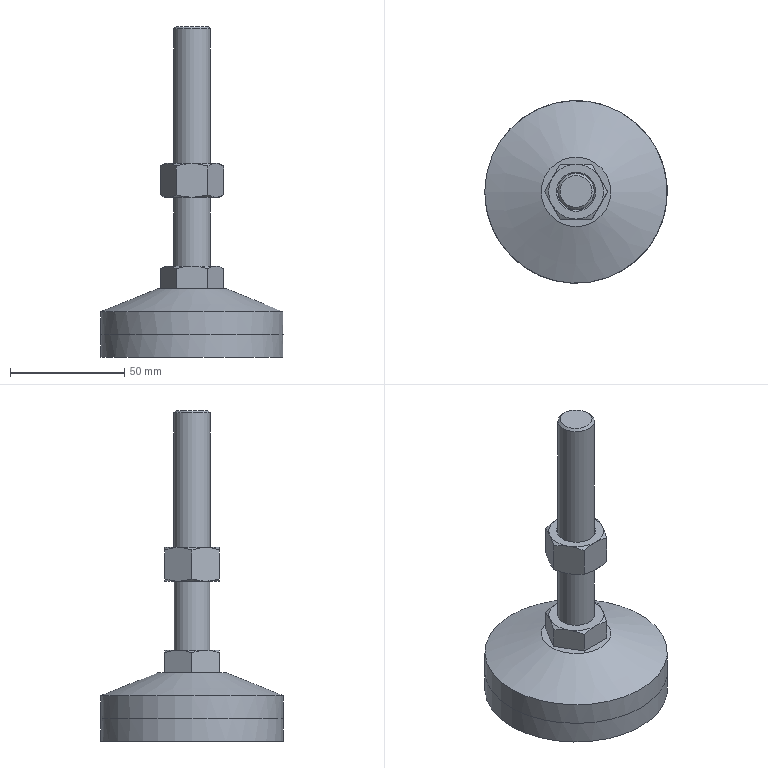Part | STEP file | 冲床-300配套压波_id614_x_t | 1 solid | 44 faces | box 80 x 80 x 145 mm | volume 156529 mm3 | cone 22 | plane 18 | cylinder 4 | commonest cylinder face diameters 16 x2 80 x2
STEP:
#1=CARTESIAN_POINT('',(1145.,255.,-875.));
#2=VERTEX_POINT('',#1);
#3=CARTESIAN_POINT('',(1185.,255.,-875.));
#4=DIRECTION('',(0.,0.,1.));
#5=DIRECTION('',(-1.,0.,0.));
#6=AXIS2_PLACEMENT_3D('',#3,#4,#5);
#7=CIRCLE('',#6,40.);
#8=EDGE_CURVE('',#2,#2,#7,.T.);
#9=ORIENTED_EDGE('',*,*,#8,.T.);
#10=EDGE_LOOP('',(#9));
#11=FACE_BOUND('',#10,.T.);
#12=CARTESIAN_POINT('',(1145.,255.,-865.));
#13=VERTEX_POINT('',#12);
#14=CARTESIAN_POINT('',(1145.,249.764,-865.));
#15=CARTESIAN_POINT('',(1145.,260.236,-865.));
#16=CARTESIAN_POINT('',(1146.041,265.47,-865.));
#17=CARTESIAN_POINT('',(1150.049,275.145,-865.));
#18=CARTESIAN_POINT('',(1153.013,279.582,-865.));
#19=CARTESIAN_POINT('',(1160.418,286.987,-865.));
#20=CARTESIAN_POINT('',(1164.855,289.951,-865.));
#21=CARTESIAN_POINT('',(1174.53,293.959,-865.));
#22=CARTESIAN_POINT('',(1179.764,295.,-865.));
#23=CARTESIAN_POINT('',(1190.236,295.,-865.));
#24=CARTESIAN_POINT('',(1195.47,293.959,-865.));
#25=CARTESIAN_POINT('',(1205.145,289.951,-865.));
#26=CARTESIAN_POINT('',(1209.582,286.987,-865.));
#27=CARTESIAN_POINT('',(1216.987,279.582,-865.));
#28=CARTESIAN_POINT('',(1219.951,275.145,-865.));
#29=CARTESIAN_POINT('',(1223.959,265.47,-865.));
#30=CARTESIAN_POINT('',(1225.,260.236,-865.));
#31=CARTESIAN_POINT('',(1225.,249.764,-865.));
#32=CARTESIAN_POINT('',(1223.959,244.53,-865.));
#33=CARTESIAN_POINT('',(1219.951,234.855,-865.));
#34=CARTESIAN_POINT('',(1216.987,230.418,-865.));
#35=CARTESIAN_POINT('',(1209.582,223.013,-865.));
#36=CARTESIAN_POINT('',(1205.145,220.049,-865.));
#37=CARTESIAN_POINT('',(1195.47,216.041,-865.));
#38=CARTESIAN_POINT('',(1190.236,215.,-865.));
#39=CARTESIAN_POINT('',(1179.764,215.,-865.));
#40=CARTESIAN_POINT('',(1174.53,216.041,-865.));
#41=CARTESIAN_POINT('',(1164.855,220.049,-865.));
#42=CARTESIAN_POINT('',(1160.418,223.013,-865.));
#43=CARTESIAN_POINT('',(1153.013,230.418,-865.));
#44=CARTESIAN_POINT('',(1150.049,234.855,-865.));
#45=CARTESIAN_POINT('',(1146.041,244.53,-865.));
#46=CARTESIAN_POINT('',(1145.,249.764,-865.));
#47=CARTESIAN_POINT('',(1145.,260.236,-865.));
#48=B_SPLINE_CURVE_WITH_KNOTS('',3,(#14,#15,#16,#17,#18,#19,#20,#21,#22,#23,#24,#25,#26,#27,#28,#29,#30,#31,#32,#33,#34,#35,#36,#37,#38,#39,#40,#41,#42,#43,#44,#45,#46,#47),.UNSPECIFIED.,.T.,.F.,(2,2,2,2,2,2,2,2,2,2,2,2,2,2,2,2,2,2,2),(-0.0625,0.,0.0625,0.125,0.1875,0.25,0.3125,0.375,0.4375,0.5,0.5625,0.625,0.6875,0.75,0.8125,0.875,0.9375,1.,1.062),.UNSPECIFIED.);
#49=EDGE_CURVE('',#13,#13,#48,.T.);
#50=ORIENTED_EDGE('',*,*,#49,.T.);
#51=EDGE_LOOP('',(#50));
#52=FACE_BOUND('',#51,.T.);
#53=CARTESIAN_POINT('',(1185.,255.,-855.));
#54=DIRECTION('',(0.,0.,-1.));
#55=DIRECTION('',(-1.,0.,0.));
#56=AXIS2_PLACEMENT_3D('',#53,#54,#55);
#57=CYLINDRICAL_SURFACE('',#56,40.);
#58=ADVANCED_FACE('',(#11,#52),#57,.T.);
#59=ORIENTED_EDGE('',*,*,#49,.F.);
#60=EDGE_LOOP('',(#59));
#61=FACE_BOUND('',#60,.T.);
#62=CARTESIAN_POINT('',(1145.,255.,-855.));
#63=VERTEX_POINT('',#62);
#64=CARTESIAN_POINT('',(1185.,255.,-855.));
#65=DIRECTION('',(0.,0.,1.));
#66=DIRECTION('',(-1.,0.,0.));
#67=AXIS2_PLACEMENT_3D('',#64,#65,#66);
#68=CIRCLE('',#67,40.);
#69=EDGE_CURVE('',#63,#63,#68,.T.);
#70=ORIENTED_EDGE('',*,*,#69,.F.);
#71=EDGE_LOOP('',(#70));
#72=FACE_BOUND('',#71,.T.);
#73=CARTESIAN_POINT('',(1185.,255.,-855.));
#74=DIRECTION('',(0.,0.,-1.));
#75=DIRECTION('',(-1.,0.,0.));
#76=AXIS2_PLACEMENT_3D('',#73,#74,#75);
#77=CYLINDRICAL_SURFACE('',#76,40.);
#78=ADVANCED_FACE('',(#61,#72),#77,.T.);
#79=ORIENTED_EDGE('',*,*,#8,.F.);
#80=EDGE_LOOP('',(#79));
#81=FACE_OUTER_BOUND('',#80,.T.);
#82=CARTESIAN_POINT('',(1185.,255.,-875.));
#83=DIRECTION('',(0.,0.,1.));
#84=DIRECTION('',(1.,0.,0.));
#85=AXIS2_PLACEMENT_3D('',#82,#83,#84);
#86=PLANE('',#85);
#87=ADVANCED_FACE('',(#81),#86,.F.);
#88=CARTESIAN_POINT('',(1169.751,255.,-845.));
#89=VERTEX_POINT('',#88);
#90=CARTESIAN_POINT('',(1185.,255.,-845.));
#91=DIRECTION('',(0.,0.,-1.));
#92=DIRECTION('',(-1.,0.,0.));
#93=AXIS2_PLACEMENT_3D('',#90,#91,#92);
#94=CIRCLE('',#93,15.249);
#95=EDGE_CURVE('',#89,#89,#94,.T.);
#96=ORIENTED_EDGE('',*,*,#95,.T.);
#97=EDGE_LOOP('',(#96));
#98=FACE_BOUND('',#97,.T.);
#99=ORIENTED_EDGE('',*,*,#69,.T.);
#100=EDGE_LOOP('',(#99));
#101=FACE_BOUND('',#100,.T.);
#102=CARTESIAN_POINT('',(1185.,255.,-855.));
#103=DIRECTION('',(0.,0.,-1.));
#104=DIRECTION('',(-1.,0.,0.));
#105=AXIS2_PLACEMENT_3D('',#102,#103,#104);
#106=CONICAL_SURFACE('',#105,40.,68.);
#107=ADVANCED_FACE('',(#98,#101),#106,.T.);
#108=CARTESIAN_POINT('',(1191.928,243.,-845.));
#109=VERTEX_POINT('',#108);
#110=CARTESIAN_POINT('',(1198.856,255.,-845.));
#111=VERTEX_POINT('',#110);
#112=CARTESIAN_POINT('',(1191.928,243.,-845.));
#113=DIRECTION('',(0.5,0.866,0.));
#114=VECTOR('',#113,1.);
#115=LINE('',#112,#114);
#116=EDGE_CURVE('',#109,#111,#115,.T.);
#117=ORIENTED_EDGE('',*,*,#116,.F.);
#118=CARTESIAN_POINT('',(1178.072,243.,-845.));
#119=VERTEX_POINT('',#118);
#120=CARTESIAN_POINT('',(1178.072,243.,-845.));
#121=DIRECTION('',(1.,0.,0.));
#122=VECTOR('',#121,1.);
#123=LINE('',#120,#122);
#124=EDGE_CURVE('',#119,#109,#123,.T.);
#125=ORIENTED_EDGE('',*,*,#124,.F.);
#126=CARTESIAN_POINT('',(1171.144,255.,-845.));
#127=VERTEX_POINT('',#126);
#128=CARTESIAN_POINT('',(1171.144,255.,-845.));
#129=DIRECTION('',(0.5,-0.866,0.));
#130=VECTOR('',#129,1.);
#131=LINE('',#128,#130);
#132=EDGE_CURVE('',#127,#119,#131,.T.);
#133=ORIENTED_EDGE('',*,*,#132,.F.);
#134=CARTESIAN_POINT('',(1178.072,267.,-845.));
#135=VERTEX_POINT('',#134);
#136=CARTESIAN_POINT('',(1178.072,267.,-845.));
#137=DIRECTION('',(-0.5,-0.866,0.));
#138=VECTOR('',#137,1.);
#139=LINE('',#136,#138);
#140=EDGE_CURVE('',#135,#127,#139,.T.);
#141=ORIENTED_EDGE('',*,*,#140,.F.);
#142=CARTESIAN_POINT('',(1191.928,267.,-845.));
#143=VERTEX_POINT('',#142);
#144=CARTESIAN_POINT('',(1191.928,267.,-845.));
#145=DIRECTION('',(-1.,0.,0.));
#146=VECTOR('',#145,1.);
#147=LINE('',#144,#146);
#148=EDGE_CURVE('',#143,#135,#147,.T.);
#149=ORIENTED_EDGE('',*,*,#148,.F.);
#150=CARTESIAN_POINT('',(1198.856,255.,-845.));
#151=DIRECTION('',(-0.5,0.866,0.));
#152=VECTOR('',#151,1.);
#153=LINE('',#150,#152);
#154=EDGE_CURVE('',#111,#143,#153,.T.);
#155=ORIENTED_EDGE('',*,*,#154,.F.);
#156=EDGE_LOOP('',(#117,#125,#133,#141,#149,#155));
#157=FACE_BOUND('',#156,.T.);
#158=ORIENTED_EDGE('',*,*,#95,.F.);
#159=EDGE_LOOP('',(#158));
#160=FACE_BOUND('',#159,.T.);
#161=CARTESIAN_POINT('',(1185.,255.,-845.));
#162=DIRECTION('',(0.,0.,-1.));
#163=DIRECTION('',(-1.,0.,0.));
#164=AXIS2_PLACEMENT_3D('',#161,#162,#163);
#165=PLANE('',#164);
#166=ADVANCED_FACE('',(#157,#160),#165,.F.);
#167=CARTESIAN_POINT('',(1178.072,243.,-836.072));
#168=VERTEX_POINT('',#167);
#169=CARTESIAN_POINT('',(1178.072,243.,-830.2));
#170=DIRECTION('',(0.,0.,1.));
#171=VECTOR('',#170,1.);
#172=LINE('',#169,#171);
#173=EDGE_CURVE('',#119,#168,#172,.T.);
#174=ORIENTED_EDGE('',*,*,#173,.T.);
#175=CARTESIAN_POINT('',(1174.608,249.,-835.));
#176=VERTEX_POINT('',#175);
#177=CARTESIAN_POINT('',(1174.608,249.,-835.));
#178=CARTESIAN_POINT('',(1175.788,246.956,-835.));
#179=CARTESIAN_POINT('',(1176.938,244.963,-835.417));
#180=CARTESIAN_POINT('',(1178.072,243.,-836.072));
#181=B_SPLINE_CURVE_WITH_KNOTS('',3,(#177,#178,#179,#180),.UNSPECIFIED.,.F.,.F.,(4,4),(0.,1.),.UNSPECIFIED.);
#182=EDGE_CURVE('',#176,#168,#181,.T.);
#183=ORIENTED_EDGE('',*,*,#182,.F.);
#184=CARTESIAN_POINT('',(1171.144,255.,-836.072));
#185=VERTEX_POINT('',#184);
#186=CARTESIAN_POINT('',(1171.144,255.,-836.072));
#187=CARTESIAN_POINT('',(1172.277,253.037,-835.417));
#188=CARTESIAN_POINT('',(1173.427,251.044,-835.));
#189=CARTESIAN_POINT('',(1174.608,249.,-835.));
#190=B_SPLINE_CURVE_WITH_KNOTS('',3,(#186,#187,#188,#189),.UNSPECIFIED.,.F.,.F.,(4,4),(0.,1.),.UNSPECIFIED.);
#191=EDGE_CURVE('',#185,#176,#190,.T.);
#192=ORIENTED_EDGE('',*,*,#191,.F.);
#193=CARTESIAN_POINT('',(1171.144,255.,-830.2));
#194=DIRECTION('',(0.,0.,1.));
#195=VECTOR('',#194,1.);
#196=LINE('',#193,#195);
#197=EDGE_CURVE('',#127,#185,#196,.T.);
#198=ORIENTED_EDGE('',*,*,#197,.F.);
#199=ORIENTED_EDGE('',*,*,#132,.T.);
#200=EDGE_LOOP('',(#174,#183,#192,#198,#199));
#201=FACE_OUTER_BOUND('',#200,.T.);
#202=CARTESIAN_POINT('',(1171.144,255.,-830.2));
#203=DIRECTION('',(-0.866,-0.5,0.));
#204=DIRECTION('',(-0.5,0.866,0.));
#205=AXIS2_PLACEMENT_3D('',#202,#203,#204);
#206=PLANE('',#205);
#207=ADVANCED_FACE('',(#201),#206,.T.);
#208=CARTESIAN_POINT('',(1191.928,243.,-836.072));
#209=VERTEX_POINT('',#208);
#210=CARTESIAN_POINT('',(1191.928,243.,-830.2));
#211=DIRECTION('',(0.,0.,1.));
#212=VECTOR('',#211,1.);
#213=LINE('',#210,#212);
#214=EDGE_CURVE('',#109,#209,#213,.T.);
#215=ORIENTED_EDGE('',*,*,#214,.T.);
#216=CARTESIAN_POINT('',(1185.,243.,-835.));
#217=VERTEX_POINT('',#216);
#218=CARTESIAN_POINT('',(1185.,243.,-835.));
#219=CARTESIAN_POINT('',(1187.361,243.,-835.));
#220=CARTESIAN_POINT('',(1189.661,243.,-835.417));
#221=CARTESIAN_POINT('',(1191.928,243.,-836.072));
#222=B_SPLINE_CURVE_WITH_KNOTS('',3,(#218,#219,#220,#221),.UNSPECIFIED.,.F.,.F.,(4,4),(0.,1.),.UNSPECIFIED.);
#223=EDGE_CURVE('',#217,#209,#222,.T.);
#224=ORIENTED_EDGE('',*,*,#223,.F.);
#225=CARTESIAN_POINT('',(1178.072,243.,-836.072));
#226=CARTESIAN_POINT('',(1180.339,243.,-835.417));
#227=CARTESIAN_POINT('',(1182.639,243.,-835.));
#228=CARTESIAN_POINT('',(1185.,243.,-835.));
#229=B_SPLINE_CURVE_WITH_KNOTS('',3,(#225,#226,#227,#228),.UNSPECIFIED.,.F.,.F.,(4,4),(0.,1.),.UNSPECIFIED.);
#230=EDGE_CURVE('',#168,#217,#229,.T.);
#231=ORIENTED_EDGE('',*,*,#230,.F.);
#232=ORIENTED_EDGE('',*,*,#173,.F.);
#233=ORIENTED_EDGE('',*,*,#124,.T.);
#234=EDGE_LOOP('',(#215,#224,#231,#232,#233));
#235=FACE_OUTER_BOUND('',#234,.T.);
#236=CARTESIAN_POINT('',(1178.072,243.,-830.2));
#237=DIRECTION('',(0.,-1.,0.));
#238=DIRECTION('',(0.,0.,1.));
#239=AXIS2_PLACEMENT_3D('',#236,#237,#238);
#240=PLANE('',#239);
#241=ADVANCED_FACE('',(#235),#240,.T.);
#242=CARTESIAN_POINT('',(1198.856,255.,-836.072));
#243=VERTEX_POINT('',#242);
#244=CARTESIAN_POINT('',(1198.856,255.,-830.2));
#245=DIRECTION('',(0.,0.,1.));
#246=VECTOR('',#245,1.);
#247=LINE('',#244,#246);
#248=EDGE_CURVE('',#111,#243,#247,.T.);
#249=ORIENTED_EDGE('',*,*,#248,.T.);
#250=CARTESIAN_POINT('',(1195.392,249.,-835.));
#251=VERTEX_POINT('',#250);
#252=CARTESIAN_POINT('',(1195.392,249.,-835.));
#253=CARTESIAN_POINT('',(1196.573,251.044,-835.));
#254=CARTESIAN_POINT('',(1197.723,253.037,-835.417));
#255=CARTESIAN_POINT('',(1198.856,255.,-836.072));
#256=B_SPLINE_CURVE_WITH_KNOTS('',3,(#252,#253,#254,#255),.UNSPECIFIED.,.F.,.F.,(4,4),(0.,1.),.UNSPECIFIED.);
#257=EDGE_CURVE('',#251,#243,#256,.T.);
#258=ORIENTED_EDGE('',*,*,#257,.F.);
#259=CARTESIAN_POINT('',(1191.928,243.,-836.072));
#260=CARTESIAN_POINT('',(1193.062,244.963,-835.417));
#261=CARTESIAN_POINT('',(1194.212,246.956,-835.));
#262=CARTESIAN_POINT('',(1195.392,249.,-835.));
#263=B_SPLINE_CURVE_WITH_KNOTS('',3,(#259,#260,#261,#262),.UNSPECIFIED.,.F.,.F.,(4,4),(0.,1.),.UNSPECIFIED.);
#264=EDGE_CURVE('',#209,#251,#263,.T.);
#265=ORIENTED_EDGE('',*,*,#264,.F.);
#266=ORIENTED_EDGE('',*,*,#214,.F.);
#267=ORIENTED_EDGE('',*,*,#116,.T.);
#268=EDGE_LOOP('',(#249,#258,#265,#266,#267));
#269=FACE_OUTER_BOUND('',#268,.T.);
#270=CARTESIAN_POINT('',(1191.928,243.,-830.2));
#271=DIRECTION('',(0.866,-0.5,0.));
#272=DIRECTION('',(-0.5,-0.866,0.));
#273=AXIS2_PLACEMENT_3D('',#270,#271,#272);
#274=PLANE('',#273);
#275=ADVANCED_FACE('',(#269),#274,.T.);
#276=CARTESIAN_POINT('',(1191.928,267.,-836.072));
#277=VERTEX_POINT('',#276);
#278=CARTESIAN_POINT('',(1191.928,267.,-830.2));
#279=DIRECTION('',(0.,0.,1.));
#280=VECTOR('',#279,1.);
#281=LINE('',#278,#280);
#282=EDGE_CURVE('',#143,#277,#281,.T.);
#283=ORIENTED_EDGE('',*,*,#282,.T.);
#284=CARTESIAN_POINT('',(1195.392,261.,-835.));
#285=VERTEX_POINT('',#284);
#286=CARTESIAN_POINT('',(1195.392,261.,-835.));
#287=CARTESIAN_POINT('',(1194.212,263.044,-835.));
#288=CARTESIAN_POINT('',(1193.062,265.037,-835.417));
#289=CARTESIAN_POINT('',(1191.928,267.,-836.072));
#290=B_SPLINE_CURVE_WITH_KNOTS('',3,(#286,#287,#288,#289),.UNSPECIFIED.,.F.,.F.,(4,4),(0.,1.),.UNSPECIFIED.);
#291=EDGE_CURVE('',#285,#277,#290,.T.);
#292=ORIENTED_EDGE('',*,*,#291,.F.);
#293=CARTESIAN_POINT('',(1198.856,255.,-836.072));
#294=CARTESIAN_POINT('',(1197.723,256.963,-835.417));
#295=CARTESIAN_POINT('',(1196.573,258.956,-835.));
#296=CARTESIAN_POINT('',(1195.392,261.,-835.));
#297=B_SPLINE_CURVE_WITH_KNOTS('',3,(#293,#294,#295,#296),.UNSPECIFIED.,.F.,.F.,(4,4),(0.,1.),.UNSPECIFIED.);
#298=EDGE_CURVE('',#243,#285,#297,.T.);
#299=ORIENTED_EDGE('',*,*,#298,.F.);
#300=ORIENTED_EDGE('',*,*,#248,.F.);
#301=ORIENTED_EDGE('',*,*,#154,.T.);
#302=EDGE_LOOP('',(#283,#292,#299,#300,#301));
#303=FACE_OUTER_BOUND('',#302,.T.);
#304=CARTESIAN_POINT('',(1198.856,255.,-830.2));
#305=DIRECTION('',(0.866,0.5,0.));
#306=DIRECTION('',(0.5,-0.866,0.));
#307=AXIS2_PLACEMENT_3D('',#304,#305,#306);
#308=PLANE('',#307);
#309=ADVANCED_FACE('',(#303),#308,.T.);
#310=CARTESIAN_POINT('',(1178.072,267.,-836.072));
#311=VERTEX_POINT('',#310);
#312=CARTESIAN_POINT('',(1178.072,267.,-830.2));
#313=DIRECTION('',(0.,0.,1.));
#314=VECTOR('',#313,1.);
#315=LINE('',#312,#314);
#316=EDGE_CURVE('',#135,#311,#315,.T.);
#317=ORIENTED_EDGE('',*,*,#316,.T.);
#318=CARTESIAN_POINT('',(1185.,267.,-835.));
#319=VERTEX_POINT('',#318);
#320=CARTESIAN_POINT('',(1185.,267.,-835.));
#321=CARTESIAN_POINT('',(1182.639,267.,-835.));
#322=CARTESIAN_POINT('',(1180.339,267.,-835.417));
#323=CARTESIAN_POINT('',(1178.072,267.,-836.072));
#324=B_SPLINE_CURVE_WITH_KNOTS('',3,(#320,#321,#322,#323),.UNSPECIFIED.,.F.,.F.,(4,4),(0.,1.),.UNSPECIFIED.);
#325=EDGE_CURVE('',#319,#311,#324,.T.);
#326=ORIENTED_EDGE('',*,*,#325,.F.);
#327=CARTESIAN_POINT('',(1191.928,267.,-836.072));
#328=CARTESIAN_POINT('',(1189.661,267.,-835.417));
#329=CARTESIAN_POINT('',(1187.361,267.,-835.));
#330=CARTESIAN_POINT('',(1185.,267.,-835.));
#331=B_SPLINE_CURVE_WITH_KNOTS('',3,(#327,#328,#329,#330),.UNSPECIFIED.,.F.,.F.,(4,4),(0.,1.),.UNSPECIFIED.);
#332=EDGE_CURVE('',#277,#319,#331,.T.);
#333=ORIENTED_EDGE('',*,*,#332,.F.);
#334=ORIENTED_EDGE('',*,*,#282,.F.);
#335=ORIENTED_EDGE('',*,*,#148,.T.);
#336=EDGE_LOOP('',(#317,#326,#333,#334,#335));
#337=FACE_OUTER_BOUND('',#336,.T.);
#338=CARTESIAN_POINT('',(1191.928,267.,-830.2));
#339=DIRECTION('',(0.,1.,0.));
#340=DIRECTION('',(0.,0.,-1.));
#341=AXIS2_PLACEMENT_3D('',#338,#339,#340);
#342=PLANE('',#341);
#343=ADVANCED_FACE('',(#337),#342,.T.);
#344=ORIENTED_EDGE('',*,*,#197,.T.);
#345=CARTESIAN_POINT('',(1174.608,261.,-835.));
#346=VERTEX_POINT('',#345);
#347=CARTESIAN_POINT('',(1174.608,261.,-835.));
#348=CARTESIAN_POINT('',(1173.427,258.956,-835.));
#349=CARTESIAN_POINT('',(1172.277,256.963,-835.417));
#350=CARTESIAN_POINT('',(1171.144,255.,-836.072));
#351=B_SPLINE_CURVE_WITH_KNOTS('',3,(#347,#348,#349,#350),.UNSPECIFIED.,.F.,.F.,(4,4),(0.,1.),.UNSPECIFIED.);
#352=EDGE_CURVE('',#346,#185,#351,.T.);
#353=ORIENTED_EDGE('',*,*,#352,.F.);
#354=CARTESIAN_POINT('',(1178.072,267.,-836.072));
#355=CARTESIAN_POINT('',(1176.938,265.037,-835.417));
#356=CARTESIAN_POINT('',(1175.788,263.044,-835.));
#357=CARTESIAN_POINT('',(1174.608,261.,-835.));
#358=B_SPLINE_CURVE_WITH_KNOTS('',3,(#354,#355,#356,#357),.UNSPECIFIED.,.F.,.F.,(4,4),(0.,1.),.UNSPECIFIED.);
#359=EDGE_CURVE('',#311,#346,#358,.T.);
#360=ORIENTED_EDGE('',*,*,#359,.F.);
#361=ORIENTED_EDGE('',*,*,#316,.F.);
#362=ORIENTED_EDGE('',*,*,#140,.T.);
#363=EDGE_LOOP('',(#344,#353,#360,#361,#362));
#364=FACE_OUTER_BOUND('',#363,.T.);
#365=CARTESIAN_POINT('',(1178.072,267.,-830.2));
#366=DIRECTION('',(-0.866,0.5,0.));
#367=DIRECTION('',(0.5,0.866,0.));
#368=AXIS2_PLACEMENT_3D('',#365,#366,#367);
#369=PLANE('',#368);
#370=ADVANCED_FACE('',(#364),#369,.T.);
#371=CARTESIAN_POINT('',(1177.,255.,-835.));
#372=VERTEX_POINT('',#371);
#373=CARTESIAN_POINT('',(1185.,255.,-835.));
#374=DIRECTION('',(0.,0.,1.));
#375=DIRECTION('',(-1.,0.,0.));
#376=AXIS2_PLACEMENT_3D('',#373,#374,#375);
#377=CIRCLE('',#376,8.);
#378=EDGE_CURVE('',#372,#372,#377,.T.);
#379=ORIENTED_EDGE('',*,*,#378,.F.);
#380=EDGE_LOOP('',(#379));
#381=FACE_BOUND('',#380,.T.);
#382=CARTESIAN_POINT('',(1185.,255.,-835.));
#383=DIRECTION('',(0.,0.,-1.));
#384=DIRECTION('',(-1.,0.,0.));
#385=AXIS2_PLACEMENT_3D('',#382,#383,#384);
#386=CIRCLE('',#385,12.);
#387=EDGE_CURVE('',#217,#176,#386,.T.);
#388=ORIENTED_EDGE('',*,*,#387,.F.);
#389=CARTESIAN_POINT('',(1185.,255.,-835.));
#390=DIRECTION('',(0.,0.,-1.));
#391=DIRECTION('',(-1.,0.,0.));
#392=AXIS2_PLACEMENT_3D('',#389,#390,#391);
#393=CIRCLE('',#392,12.);
#394=EDGE_CURVE('',#251,#217,#393,.T.);
#395=ORIENTED_EDGE('',*,*,#394,.F.);
#396=CARTESIAN_POINT('',(1185.,255.,-835.));
#397=DIRECTION('',(0.,0.,-1.));
#398=DIRECTION('',(-1.,0.,0.));
#399=AXIS2_PLACEMENT_3D('',#396,#397,#398);
#400=CIRCLE('',#399,12.);
#401=EDGE_CURVE('',#285,#251,#400,.T.);
#402=ORIENTED_EDGE('',*,*,#401,.F.);
#403=CARTESIAN_POINT('',(1185.,255.,-835.));
#404=DIRECTION('',(0.,0.,-1.));
#405=DIRECTION('',(-1.,0.,0.));
#406=AXIS2_PLACEMENT_3D('',#403,#404,#405);
#407=CIRCLE('',#406,12.);
#408=EDGE_CURVE('',#319,#285,#407,.T.);
#409=ORIENTED_EDGE('',*,*,#408,.F.);
#410=CARTESIAN_POINT('',(1185.,255.,-835.));
#411=DIRECTION('',(0.,0.,-1.));
#412=DIRECTION('',(-1.,0.,0.));
#413=AXIS2_PLACEMENT_3D('',#410,#411,#412);
#414=CIRCLE('',#413,12.);
#415=EDGE_CURVE('',#346,#319,#414,.T.);
#416=ORIENTED_EDGE('',*,*,#415,.F.);
#417=CARTESIAN_POINT('',(1185.,255.,-835.));
#418=DIRECTION('',(0.,0.,-1.));
#419=DIRECTION('',(-1.,0.,0.));
#420=AXIS2_PLACEMENT_3D('',#417,#418,#419);
#421=CIRCLE('',#420,12.);
#422=EDGE_CURVE('',#176,#346,#421,.T.);
#423=ORIENTED_EDGE('',*,*,#422,.F.);
#424=EDGE_LOOP('',(#388,#395,#402,#409,#416,#423));
#425=FACE_BOUND('',#424,.T.);
#426=CARTESIAN_POINT('',(1178.072,243.,-835.));
#427=DIRECTION('',(0.,0.,-1.));
#428=DIRECTION('',(-1.,0.,0.));
#429=AXIS2_PLACEMENT_3D('',#426,#427,#428);
#430=PLANE('',#429);
#431=ADVANCED_FACE('',(#381,#425),#430,.F.);
#432=ORIENTED_EDGE('',*,*,#325,.T.);
#433=ORIENTED_EDGE('',*,*,#359,.T.);
#434=ORIENTED_EDGE('',*,*,#415,.T.);
#435=EDGE_LOOP('',(#432,#433,#434));
#436=FACE_OUTER_BOUND('',#435,.T.);
#437=CARTESIAN_POINT('',(1185.,255.,-835.));
#438=DIRECTION('',(0.,0.,-1.));
#439=DIRECTION('',(-1.,0.,0.));
#440=AXIS2_PLACEMENT_3D('',#437,#438,#439);
#441=CONICAL_SURFACE('',#440,12.,60.);
#442=ADVANCED_FACE('',(#436),#441,.T.);
#443=ORIENTED_EDGE('',*,*,#191,.T.);
#444=ORIENTED_EDGE('',*,*,#422,.T.);
#445=ORIENTED_EDGE('',*,*,#352,.T.);
#446=EDGE_LOOP('',(#443,#444,#445));
#447=FACE_OUTER_BOUND('',#446,.T.);
#448=CARTESIAN_POINT('',(1185.,255.,-835.));
#449=DIRECTION('',(0.,0.,-1.));
#450=DIRECTION('',(-1.,0.,0.));
#451=AXIS2_PLACEMENT_3D('',#448,#449,#450);
#452=CONICAL_SURFACE('',#451,12.,60.);
#453=ADVANCED_FACE('',(#447),#452,.T.);
#454=ORIENTED_EDGE('',*,*,#291,.T.);
#455=ORIENTED_EDGE('',*,*,#332,.T.);
#456=ORIENTED_EDGE('',*,*,#408,.T.);
#457=EDGE_LOOP('',(#454,#455,#456));
#458=FACE_OUTER_BOUND('',#457,.T.);
#459=CARTESIAN_POINT('',(1185.,255.,-835.));
#460=DIRECTION('',(0.,0.,-1.));
#461=DIRECTION('',(-1.,0.,0.));
#462=AXIS2_PLACEMENT_3D('',#459,#460,#461);
#463=CONICAL_SURFACE('',#462,12.,60.);
#464=ADVANCED_FACE('',(#458),#463,.T.);
#465=ORIENTED_EDGE('',*,*,#257,.T.);
#466=ORIENTED_EDGE('',*,*,#298,.T.);
#467=ORIENTED_EDGE('',*,*,#401,.T.);
#468=EDGE_LOOP('',(#465,#466,#467));
#469=FACE_OUTER_BOUND('',#468,.T.);
#470=CARTESIAN_POINT('',(1185.,255.,-835.));
#471=DIRECTION('',(0.,0.,-1.));
#472=DIRECTION('',(-1.,0.,0.));
#473=AXIS2_PLACEMENT_3D('',#470,#471,#472);
#474=CONICAL_SURFACE('',#473,12.,60.);
#475=ADVANCED_FACE('',(#469),#474,.T.);
#476=ORIENTED_EDGE('',*,*,#264,.T.);
#477=ORIENTED_EDGE('',*,*,#394,.T.);
#478=ORIENTED_EDGE('',*,*,#223,.T.);
#479=EDGE_LOOP('',(#476,#477,#478));
#480=FACE_OUTER_BOUND('',#479,.T.);
#481=CARTESIAN_POINT('',(1185.,255.,-835.));
#482=DIRECTION('',(0.,0.,-1.));
#483=DIRECTION('',(-1.,0.,0.));
#484=AXIS2_PLACEMENT_3D('',#481,#482,#483);
#485=CONICAL_SURFACE('',#484,12.,60.);
#486=ADVANCED_FACE('',(#480),#485,.T.);
#487=ORIENTED_EDGE('',*,*,#230,.T.);
#488=ORIENTED_EDGE('',*,*,#387,.T.);
#489=ORIENTED_EDGE('',*,*,#182,.T.);
#490=EDGE_LOOP('',(#487,#488,#489));
#491=FACE_OUTER_BOUND('',#490,.T.);
#492=CARTESIAN_POINT('',(1185.,255.,-835.));
#493=DIRECTION('',(0.,0.,-1.));
#494=DIRECTION('',(-1.,0.,0.));
#495=AXIS2_PLACEMENT_3D('',#492,#493,#494);
#496=CONICAL_SURFACE('',#495,12.,60.);
#497=ADVANCED_FACE('',(#491),#496,.T.);
#498=CARTESIAN_POINT('',(1177.,255.,-804.232));
#499=VERTEX_POINT('',#498);
#500=CARTESIAN_POINT('',(1185.,255.,-804.232));
#501=DIRECTION('',(0.,0.,1.));
#502=DIRECTION('',(-1.,0.,0.));
#503=AXIS2_PLACEMENT_3D('',#500,#501,#502);
#504=CIRCLE('',#503,8.);
#505=EDGE_CURVE('',#499,#499,#504,.T.);
#506=ORIENTED_EDGE('',*,*,#505,.F.);
#507=EDGE_LOOP('',(#506));
#508=FACE_BOUND('',#507,.T.);
#509=ORIENTED_EDGE('',*,*,#378,.T.);
#510=EDGE_LOOP('',(#509));
#511=FACE_BOUND('',#510,.T.);
#512=CARTESIAN_POINT('',(1185.,255.,-740.));
#513=DIRECTION('',(0.,0.,-1.));
#514=DIRECTION('',(-1.,0.,0.));
#515=AXIS2_PLACEMENT_3D('',#512,#513,#514);
#516=CYLINDRICAL_SURFACE('',#515,8.);
#517=ADVANCED_FACE('',(#508,#511),#516,.T.);
#518=CARTESIAN_POINT('',(1191.928,243.,-791.072));
#519=VERTEX_POINT('',#518);
#520=CARTESIAN_POINT('',(1191.928,243.,-803.728));
#521=VERTEX_POINT('',#520);
#522=CARTESIAN_POINT('',(1191.928,243.,-804.8));
#523=DIRECTION('',(0.,0.,-1.));
#524=VECTOR('',#523,1.);
#525=LINE('',#522,#524);
#526=EDGE_CURVE('',#519,#521,#525,.T.);
#527=ORIENTED_EDGE('',*,*,#526,.T.);
#528=CARTESIAN_POINT('',(1195.392,249.,-804.8));
#529=VERTEX_POINT('',#528);
#530=CARTESIAN_POINT('',(1195.392,249.,-804.8));
#531=CARTESIAN_POINT('',(1194.212,246.956,-804.8));
#532=CARTESIAN_POINT('',(1193.062,244.963,-804.383));
#533=CARTESIAN_POINT('',(1191.928,243.,-803.728));
#534=B_SPLINE_CURVE_WITH_KNOTS('',3,(#530,#531,#532,#533),.UNSPECIFIED.,.F.,.F.,(4,4),(0.,1.),.UNSPECIFIED.);
#535=EDGE_CURVE('',#529,#521,#534,.T.);
#536=ORIENTED_EDGE('',*,*,#535,.F.);
#537=CARTESIAN_POINT('',(1198.856,255.,-803.728));
#538=VERTEX_POINT('',#537);
#539=CARTESIAN_POINT('',(1198.856,255.,-803.728));
#540=CARTESIAN_POINT('',(1197.726,253.042,-804.381));
#541=CARTESIAN_POINT('',(1196.568,251.037,-804.8));
#542=CARTESIAN_POINT('',(1195.392,249.,-804.8));
#543=B_SPLINE_CURVE_WITH_KNOTS('',3,(#539,#540,#541,#542),.UNSPECIFIED.,.F.,.F.,(4,4),(0.,1.),.UNSPECIFIED.);
#544=EDGE_CURVE('',#538,#529,#543,.T.);
#545=ORIENTED_EDGE('',*,*,#544,.F.);
#546=CARTESIAN_POINT('',(1198.856,255.,-791.072));
#547=VERTEX_POINT('',#546);
#548=CARTESIAN_POINT('',(1198.856,255.,-804.8));
#549=DIRECTION('',(0.,0.,-1.));
#550=VECTOR('',#549,1.);
#551=LINE('',#548,#550);
#552=EDGE_CURVE('',#547,#538,#551,.T.);
#553=ORIENTED_EDGE('',*,*,#552,.F.);
#554=CARTESIAN_POINT('',(1195.392,249.,-790.));
#555=VERTEX_POINT('',#554);
#556=CARTESIAN_POINT('',(1198.856,255.,-791.072));
#557=CARTESIAN_POINT('',(1197.726,253.042,-790.419));
#558=CARTESIAN_POINT('',(1196.568,251.037,-790.));
#559=CARTESIAN_POINT('',(1195.392,249.,-790.));
#560=B_SPLINE_CURVE_WITH_KNOTS('',3,(#556,#557,#558,#559),.UNSPECIFIED.,.F.,.F.,(4,4),(0.,1.),.UNSPECIFIED.);
#561=EDGE_CURVE('',#547,#555,#560,.T.);
#562=ORIENTED_EDGE('',*,*,#561,.T.);
#563=CARTESIAN_POINT('',(1195.392,249.,-790.));
#564=CARTESIAN_POINT('',(1194.212,246.956,-790.));
#565=CARTESIAN_POINT('',(1193.062,244.963,-790.417));
#566=CARTESIAN_POINT('',(1191.928,243.,-791.072));
#567=B_SPLINE_CURVE_WITH_KNOTS('',3,(#563,#564,#565,#566),.UNSPECIFIED.,.F.,.F.,(4,4),(0.,1.),.UNSPECIFIED.);
#568=EDGE_CURVE('',#555,#519,#567,.T.);
#569=ORIENTED_EDGE('',*,*,#568,.T.);
#570=EDGE_LOOP('',(#527,#536,#545,#553,#562,#569));
#571=FACE_OUTER_BOUND('',#570,.T.);
#572=CARTESIAN_POINT('',(1198.856,255.,-804.8));
#573=DIRECTION('',(0.866,-0.5,0.));
#574=DIRECTION('',(0.5,0.866,0.));
#575=AXIS2_PLACEMENT_3D('',#572,#573,#574);
#576=PLANE('',#575);
#577=ADVANCED_FACE('',(#571),#576,.T.);
#578=CARTESIAN_POINT('',(1178.072,243.,-791.072));
#579=VERTEX_POINT('',#578);
#580=CARTESIAN_POINT('',(1178.072,243.,-803.728));
#581=VERTEX_POINT('',#580);
#582=CARTESIAN_POINT('',(1178.072,243.,-804.8));
#583=DIRECTION('',(0.,0.,-1.));
#584=VECTOR('',#583,1.);
#585=LINE('',#582,#584);
#586=EDGE_CURVE('',#579,#581,#585,.T.);
#587=ORIENTED_EDGE('',*,*,#586,.T.);
#588=CARTESIAN_POINT('',(1185.,243.,-804.8));
#589=VERTEX_POINT('',#588);
#590=CARTESIAN_POINT('',(1185.,243.,-804.8));
#591=CARTESIAN_POINT('',(1182.657,243.,-804.8));
#592=CARTESIAN_POINT('',(1180.312,243.,-804.375));
#593=CARTESIAN_POINT('',(1178.072,243.,-803.728));
#594=B_SPLINE_CURVE_WITH_KNOTS('',3,(#590,#591,#592,#593),.UNSPECIFIED.,.F.,.F.,(4,4),(0.,1.),.UNSPECIFIED.);
#595=EDGE_CURVE('',#589,#581,#594,.T.);
#596=ORIENTED_EDGE('',*,*,#595,.F.);
#597=CARTESIAN_POINT('',(1191.928,243.,-803.728));
#598=CARTESIAN_POINT('',(1189.675,243.,-804.379));
#599=CARTESIAN_POINT('',(1187.342,243.,-804.8));
#600=CARTESIAN_POINT('',(1185.,243.,-804.8));
#601=B_SPLINE_CURVE_WITH_KNOTS('',3,(#597,#598,#599,#600),.UNSPECIFIED.,.F.,.F.,(4,4),(0.,1.),.UNSPECIFIED.);
#602=EDGE_CURVE('',#521,#589,#601,.T.);
#603=ORIENTED_EDGE('',*,*,#602,.F.);
#604=ORIENTED_EDGE('',*,*,#526,.F.);
#605=CARTESIAN_POINT('',(1185.,243.,-790.));
#606=VERTEX_POINT('',#605);
#607=CARTESIAN_POINT('',(1191.928,243.,-791.072));
#608=CARTESIAN_POINT('',(1189.675,243.,-790.421));
#609=CARTESIAN_POINT('',(1187.342,243.,-790.));
#610=CARTESIAN_POINT('',(1185.,243.,-790.));
#611=B_SPLINE_CURVE_WITH_KNOTS('',3,(#607,#608,#609,#610),.UNSPECIFIED.,.F.,.F.,(4,4),(0.,1.),.UNSPECIFIED.);
#612=EDGE_CURVE('',#519,#606,#611,.T.);
#613=ORIENTED_EDGE('',*,*,#612,.T.);
#614=CARTESIAN_POINT('',(1185.,243.,-790.));
#615=CARTESIAN_POINT('',(1182.657,243.,-790.));
#616=CARTESIAN_POINT('',(1180.312,243.,-790.425));
#617=CARTESIAN_POINT('',(1178.072,243.,-791.072));
#618=B_SPLINE_CURVE_WITH_KNOTS('',3,(#614,#615,#616,#617),.UNSPECIFIED.,.F.,.F.,(4,4),(0.,1.),.UNSPECIFIED.);
#619=EDGE_CURVE('',#606,#579,#618,.T.);
#620=ORIENTED_EDGE('',*,*,#619,.T.);
#621=EDGE_LOOP('',(#587,#596,#603,#604,#613,#620));
#622=FACE_OUTER_BOUND('',#621,.T.);
#623=CARTESIAN_POINT('',(1191.928,243.,-804.8));
#624=DIRECTION('',(0.,-1.,0.));
#625=DIRECTION('',(0.,0.,-1.));
#626=AXIS2_PLACEMENT_3D('',#623,#624,#625);
#627=PLANE('',#626);
#628=ADVANCED_FACE('',(#622),#627,.T.);
#629=CARTESIAN_POINT('',(1171.144,255.,-791.072));
#630=VERTEX_POINT('',#629);
#631=CARTESIAN_POINT('',(1171.144,255.,-803.728));
#632=VERTEX_POINT('',#631);
#633=CARTESIAN_POINT('',(1171.144,255.,-804.8));
#634=DIRECTION('',(0.,0.,-1.));
#635=VECTOR('',#634,1.);
#636=LINE('',#633,#635);
#637=EDGE_CURVE('',#630,#632,#636,.T.);
#638=ORIENTED_EDGE('',*,*,#637,.T.);
#639=CARTESIAN_POINT('',(1174.608,249.,-804.8));
#640=VERTEX_POINT('',#639);
#641=CARTESIAN_POINT('',(1174.608,249.,-804.8));
#642=CARTESIAN_POINT('',(1173.427,251.044,-804.8));
#643=CARTESIAN_POINT('',(1172.277,253.037,-804.383));
#644=CARTESIAN_POINT('',(1171.144,255.,-803.728));
#645=B_SPLINE_CURVE_WITH_KNOTS('',3,(#641,#642,#643,#644),.UNSPECIFIED.,.F.,.F.,(4,4),(0.,1.),.UNSPECIFIED.);
#646=EDGE_CURVE('',#640,#632,#645,.T.);
#647=ORIENTED_EDGE('',*,*,#646,.F.);
#648=CARTESIAN_POINT('',(1178.072,243.,-803.728));
#649=CARTESIAN_POINT('',(1176.941,244.958,-804.381));
#650=CARTESIAN_POINT('',(1175.784,246.963,-804.8));
#651=CARTESIAN_POINT('',(1174.608,249.,-804.8));
#652=B_SPLINE_CURVE_WITH_KNOTS('',3,(#648,#649,#650,#651),.UNSPECIFIED.,.F.,.F.,(4,4),(0.,1.),.UNSPECIFIED.);
#653=EDGE_CURVE('',#581,#640,#652,.T.);
#654=ORIENTED_EDGE('',*,*,#653,.F.);
#655=ORIENTED_EDGE('',*,*,#586,.F.);
#656=CARTESIAN_POINT('',(1174.608,249.,-790.));
#657=VERTEX_POINT('',#656);
#658=CARTESIAN_POINT('',(1178.072,243.,-791.072));
#659=CARTESIAN_POINT('',(1176.941,244.958,-790.419));
#660=CARTESIAN_POINT('',(1175.784,246.963,-790.));
#661=CARTESIAN_POINT('',(1174.608,249.,-790.));
#662=B_SPLINE_CURVE_WITH_KNOTS('',3,(#658,#659,#660,#661),.UNSPECIFIED.,.F.,.F.,(4,4),(0.,1.),.UNSPECIFIED.);
#663=EDGE_CURVE('',#579,#657,#662,.T.);
#664=ORIENTED_EDGE('',*,*,#663,.T.);
#665=CARTESIAN_POINT('',(1174.608,249.,-790.));
#666=CARTESIAN_POINT('',(1173.427,251.044,-790.));
#667=CARTESIAN_POINT('',(1172.277,253.037,-790.417));
#668=CARTESIAN_POINT('',(1171.144,255.,-791.072));
#669=B_SPLINE_CURVE_WITH_KNOTS('',3,(#665,#666,#667,#668),.UNSPECIFIED.,.F.,.F.,(4,4),(0.,1.),.UNSPECIFIED.);
#670=EDGE_CURVE('',#657,#630,#669,.T.);
#671=ORIENTED_EDGE('',*,*,#670,.T.);
#672=EDGE_LOOP('',(#638,#647,#654,#655,#664,#671));
#673=FACE_OUTER_BOUND('',#672,.T.);
#674=CARTESIAN_POINT('',(1178.072,243.,-804.8));
#675=DIRECTION('',(-0.866,-0.5,0.));
#676=DIRECTION('',(0.5,-0.866,0.));
#677=AXIS2_PLACEMENT_3D('',#674,#675,#676);
#678=PLANE('',#677);
#679=ADVANCED_FACE('',(#673),#678,.T.);
#680=CARTESIAN_POINT('',(1178.072,267.,-791.072));
#681=VERTEX_POINT('',#680);
#682=CARTESIAN_POINT('',(1178.072,267.,-803.728));
#683=VERTEX_POINT('',#682);
#684=CARTESIAN_POINT('',(1178.072,267.,-804.8));
#685=DIRECTION('',(0.,0.,-1.));
#686=VECTOR('',#685,1.);
#687=LINE('',#684,#686);
#688=EDGE_CURVE('',#681,#683,#687,.T.);
#689=ORIENTED_EDGE('',*,*,#688,.T.);
#690=CARTESIAN_POINT('',(1174.608,261.,-804.8));
#691=VERTEX_POINT('',#690);
#692=CARTESIAN_POINT('',(1174.608,261.,-804.8));
#693=CARTESIAN_POINT('',(1175.788,263.044,-804.8));
#694=CARTESIAN_POINT('',(1176.938,265.037,-804.383));
#695=CARTESIAN_POINT('',(1178.072,267.,-803.728));
#696=B_SPLINE_CURVE_WITH_KNOTS('',3,(#692,#693,#694,#695),.UNSPECIFIED.,.F.,.F.,(4,4),(0.,1.),.UNSPECIFIED.);
#697=EDGE_CURVE('',#691,#683,#696,.T.);
#698=ORIENTED_EDGE('',*,*,#697,.F.);
#699=CARTESIAN_POINT('',(1171.144,255.,-803.728));
#700=CARTESIAN_POINT('',(1172.274,256.958,-804.381));
#701=CARTESIAN_POINT('',(1173.432,258.963,-804.8));
#702=CARTESIAN_POINT('',(1174.608,261.,-804.8));
#703=B_SPLINE_CURVE_WITH_KNOTS('',3,(#699,#700,#701,#702),.UNSPECIFIED.,.F.,.F.,(4,4),(0.,1.),.UNSPECIFIED.);
#704=EDGE_CURVE('',#632,#691,#703,.T.);
#705=ORIENTED_EDGE('',*,*,#704,.F.);
#706=ORIENTED_EDGE('',*,*,#637,.F.);
#707=CARTESIAN_POINT('',(1174.608,261.,-790.));
#708=VERTEX_POINT('',#707);
#709=CARTESIAN_POINT('',(1171.144,255.,-791.072));
#710=CARTESIAN_POINT('',(1172.274,256.958,-790.419));
#711=CARTESIAN_POINT('',(1173.432,258.963,-790.));
#712=CARTESIAN_POINT('',(1174.608,261.,-790.));
#713=B_SPLINE_CURVE_WITH_KNOTS('',3,(#709,#710,#711,#712),.UNSPECIFIED.,.F.,.F.,(4,4),(0.,1.),.UNSPECIFIED.);
#714=EDGE_CURVE('',#630,#708,#713,.T.);
#715=ORIENTED_EDGE('',*,*,#714,.T.);
#716=CARTESIAN_POINT('',(1174.608,261.,-790.));
#717=CARTESIAN_POINT('',(1175.788,263.044,-790.));
#718=CARTESIAN_POINT('',(1176.938,265.037,-790.417));
#719=CARTESIAN_POINT('',(1178.072,267.,-791.072));
#720=B_SPLINE_CURVE_WITH_KNOTS('',3,(#716,#717,#718,#719),.UNSPECIFIED.,.F.,.F.,(4,4),(0.,1.),.UNSPECIFIED.);
#721=EDGE_CURVE('',#708,#681,#720,.T.);
#722=ORIENTED_EDGE('',*,*,#721,.T.);
#723=EDGE_LOOP('',(#689,#698,#705,#706,#715,#722));
#724=FACE_OUTER_BOUND('',#723,.T.);
#725=CARTESIAN_POINT('',(1171.144,255.,-804.8));
#726=DIRECTION('',(-0.866,0.5,0.));
#727=DIRECTION('',(-0.5,-0.866,0.));
#728=AXIS2_PLACEMENT_3D('',#725,#726,#727);
#729=PLANE('',#728);
#730=ADVANCED_FACE('',(#724),#729,.T.);
#731=CARTESIAN_POINT('',(1191.928,267.,-791.072));
#732=VERTEX_POINT('',#731);
#733=CARTESIAN_POINT('',(1191.928,267.,-803.728));
#734=VERTEX_POINT('',#733);
#735=CARTESIAN_POINT('',(1191.928,267.,-804.8));
#736=DIRECTION('',(0.,0.,-1.));
#737=VECTOR('',#736,1.);
#738=LINE('',#735,#737);
#739=EDGE_CURVE('',#732,#734,#738,.T.);
#740=ORIENTED_EDGE('',*,*,#739,.T.);
#741=CARTESIAN_POINT('',(1185.,267.,-804.8));
#742=VERTEX_POINT('',#741);
#743=CARTESIAN_POINT('',(1185.,267.,-804.8));
#744=CARTESIAN_POINT('',(1187.342,267.,-804.8));
#745=CARTESIAN_POINT('',(1189.675,267.,-804.379));
#746=CARTESIAN_POINT('',(1191.928,267.,-803.728));
#747=B_SPLINE_CURVE_WITH_KNOTS('',3,(#743,#744,#745,#746),.UNSPECIFIED.,.F.,.F.,(4,4),(0.,1.),.UNSPECIFIED.);
#748=EDGE_CURVE('',#742,#734,#747,.T.);
#749=ORIENTED_EDGE('',*,*,#748,.F.);
#750=CARTESIAN_POINT('',(1178.072,267.,-803.728));
#751=CARTESIAN_POINT('',(1180.312,267.,-804.375));
#752=CARTESIAN_POINT('',(1182.657,267.,-804.8));
#753=CARTESIAN_POINT('',(1185.,267.,-804.8));
#754=B_SPLINE_CURVE_WITH_KNOTS('',3,(#750,#751,#752,#753),.UNSPECIFIED.,.F.,.F.,(4,4),(0.,1.),.UNSPECIFIED.);
#755=EDGE_CURVE('',#683,#742,#754,.T.);
#756=ORIENTED_EDGE('',*,*,#755,.F.);
#757=ORIENTED_EDGE('',*,*,#688,.F.);
#758=CARTESIAN_POINT('',(1185.,267.,-790.));
#759=VERTEX_POINT('',#758);
#760=CARTESIAN_POINT('',(1178.072,267.,-791.072));
#761=CARTESIAN_POINT('',(1180.312,267.,-790.425));
#762=CARTESIAN_POINT('',(1182.657,267.,-790.));
#763=CARTESIAN_POINT('',(1185.,267.,-790.));
#764=B_SPLINE_CURVE_WITH_KNOTS('',3,(#760,#761,#762,#763),.UNSPECIFIED.,.F.,.F.,(4,4),(0.,1.),.UNSPECIFIED.);
#765=EDGE_CURVE('',#681,#759,#764,.T.);
#766=ORIENTED_EDGE('',*,*,#765,.T.);
#767=CARTESIAN_POINT('',(1185.,267.,-790.));
#768=CARTESIAN_POINT('',(1187.342,267.,-790.));
#769=CARTESIAN_POINT('',(1189.675,267.,-790.421));
#770=CARTESIAN_POINT('',(1191.928,267.,-791.072));
#771=B_SPLINE_CURVE_WITH_KNOTS('',3,(#767,#768,#769,#770),.UNSPECIFIED.,.F.,.F.,(4,4),(0.,1.),.UNSPECIFIED.);
#772=EDGE_CURVE('',#759,#732,#771,.T.);
#773=ORIENTED_EDGE('',*,*,#772,.T.);
#774=EDGE_LOOP('',(#740,#749,#756,#757,#766,#773));
#775=FACE_OUTER_BOUND('',#774,.T.);
#776=CARTESIAN_POINT('',(1178.072,267.,-804.8));
#777=DIRECTION('',(0.,1.,0.));
#778=DIRECTION('',(0.,0.,1.));
#779=AXIS2_PLACEMENT_3D('',#776,#777,#778);
#780=PLANE('',#779);
#781=ADVANCED_FACE('',(#775),#780,.T.);
#782=ORIENTED_EDGE('',*,*,#552,.T.);
#783=CARTESIAN_POINT('',(1195.392,261.,-804.8));
#784=VERTEX_POINT('',#783);
#785=CARTESIAN_POINT('',(1195.392,261.,-804.8));
#786=CARTESIAN_POINT('',(1196.573,258.956,-804.8));
#787=CARTESIAN_POINT('',(1197.723,256.963,-804.383));
#788=CARTESIAN_POINT('',(1198.856,255.,-803.728));
#789=B_SPLINE_CURVE_WITH_KNOTS('',3,(#785,#786,#787,#788),.UNSPECIFIED.,.F.,.F.,(4,4),(0.,1.),.UNSPECIFIED.);
#790=EDGE_CURVE('',#784,#538,#789,.T.);
#791=ORIENTED_EDGE('',*,*,#790,.F.);
#792=CARTESIAN_POINT('',(1191.928,267.,-803.728));
#793=CARTESIAN_POINT('',(1193.059,265.042,-804.381));
#794=CARTESIAN_POINT('',(1194.216,263.037,-804.8));
#795=CARTESIAN_POINT('',(1195.392,261.,-804.8));
#796=B_SPLINE_CURVE_WITH_KNOTS('',3,(#792,#793,#794,#795),.UNSPECIFIED.,.F.,.F.,(4,4),(0.,1.),.UNSPECIFIED.);
#797=EDGE_CURVE('',#734,#784,#796,.T.);
#798=ORIENTED_EDGE('',*,*,#797,.F.);
#799=ORIENTED_EDGE('',*,*,#739,.F.);
#800=CARTESIAN_POINT('',(1195.392,261.,-790.));
#801=VERTEX_POINT('',#800);
#802=CARTESIAN_POINT('',(1191.928,267.,-791.072));
#803=CARTESIAN_POINT('',(1193.059,265.042,-790.419));
#804=CARTESIAN_POINT('',(1194.216,263.037,-790.));
#805=CARTESIAN_POINT('',(1195.392,261.,-790.));
#806=B_SPLINE_CURVE_WITH_KNOTS('',3,(#802,#803,#804,#805),.UNSPECIFIED.,.F.,.F.,(4,4),(0.,1.),.UNSPECIFIED.);
#807=EDGE_CURVE('',#732,#801,#806,.T.);
#808=ORIENTED_EDGE('',*,*,#807,.T.);
#809=CARTESIAN_POINT('',(1195.392,261.,-790.));
#810=CARTESIAN_POINT('',(1196.573,258.956,-790.));
#811=CARTESIAN_POINT('',(1197.723,256.963,-790.417));
#812=CARTESIAN_POINT('',(1198.856,255.,-791.072));
#813=B_SPLINE_CURVE_WITH_KNOTS('',3,(#809,#810,#811,#812),.UNSPECIFIED.,.F.,.F.,(4,4),(0.,1.),.UNSPECIFIED.);
#814=EDGE_CURVE('',#801,#547,#813,.T.);
#815=ORIENTED_EDGE('',*,*,#814,.T.);
#816=EDGE_LOOP('',(#782,#791,#798,#799,#808,#815));
#817=FACE_OUTER_BOUND('',#816,.T.);
#818=CARTESIAN_POINT('',(1191.928,267.,-804.8));
#819=DIRECTION('',(0.866,0.5,0.));
#820=DIRECTION('',(-0.5,0.866,0.));
#821=AXIS2_PLACEMENT_3D('',#818,#819,#820);
#822=PLANE('',#821);
#823=ADVANCED_FACE('',(#817),#822,.T.);
#824=CARTESIAN_POINT('',(1193.568,255.,-790.));
#825=VERTEX_POINT('',#824);
#826=CARTESIAN_POINT('',(1185.,255.,-790.));
#827=DIRECTION('',(0.,0.,-1.));
#828=DIRECTION('',(1.,0.,0.));
#829=AXIS2_PLACEMENT_3D('',#826,#827,#828);
#830=CIRCLE('',#829,8.568);
#831=EDGE_CURVE('',#825,#825,#830,.T.);
#832=ORIENTED_EDGE('',*,*,#831,.T.);
#833=EDGE_LOOP('',(#832));
#834=FACE_BOUND('',#833,.T.);
#835=CARTESIAN_POINT('',(1185.,255.,-790.));
#836=DIRECTION('',(0.,0.,1.));
#837=DIRECTION('',(1.,0.,0.));
#838=AXIS2_PLACEMENT_3D('',#835,#836,#837);
#839=CIRCLE('',#838,12.);
#840=EDGE_CURVE('',#555,#801,#839,.T.);
#841=ORIENTED_EDGE('',*,*,#840,.T.);
#842=CARTESIAN_POINT('',(1185.,255.,-790.));
#843=DIRECTION('',(0.,0.,1.));
#844=DIRECTION('',(1.,0.,0.));
#845=AXIS2_PLACEMENT_3D('',#842,#843,#844);
#846=CIRCLE('',#845,12.);
#847=EDGE_CURVE('',#801,#759,#846,.T.);
#848=ORIENTED_EDGE('',*,*,#847,.T.);
#849=CARTESIAN_POINT('',(1185.,255.,-790.));
#850=DIRECTION('',(0.,0.,1.));
#851=DIRECTION('',(1.,0.,0.));
#852=AXIS2_PLACEMENT_3D('',#849,#850,#851);
#853=CIRCLE('',#852,12.);
#854=EDGE_CURVE('',#759,#708,#853,.T.);
#855=ORIENTED_EDGE('',*,*,#854,.T.);
#856=CARTESIAN_POINT('',(1185.,255.,-790.));
#857=DIRECTION('',(0.,0.,1.));
#858=DIRECTION('',(1.,0.,0.));
#859=AXIS2_PLACEMENT_3D('',#856,#857,#858);
#860=CIRCLE('',#859,12.);
#861=EDGE_CURVE('',#708,#657,#860,.T.);
#862=ORIENTED_EDGE('',*,*,#861,.T.);
#863=CARTESIAN_POINT('',(1185.,255.,-790.));
#864=DIRECTION('',(0.,0.,1.));
#865=DIRECTION('',(1.,0.,0.));
#866=AXIS2_PLACEMENT_3D('',#863,#864,#865);
#867=CIRCLE('',#866,12.);
#868=EDGE_CURVE('',#657,#606,#867,.T.);
#869=ORIENTED_EDGE('',*,*,#868,.T.);
#870=CARTESIAN_POINT('',(1185.,255.,-790.));
#871=DIRECTION('',(0.,0.,1.));
#872=DIRECTION('',(1.,0.,0.));
#873=AXIS2_PLACEMENT_3D('',#870,#871,#872);
#874=CIRCLE('',#873,12.);
#875=EDGE_CURVE('',#606,#555,#874,.T.);
#876=ORIENTED_EDGE('',*,*,#875,.T.);
#877=EDGE_LOOP('',(#841,#848,#855,#862,#869,#876));
#878=FACE_BOUND('',#877,.T.);
#879=CARTESIAN_POINT('',(1191.928,243.,-790.));
#880=DIRECTION('',(0.,0.,1.));
#881=DIRECTION('',(1.,0.,0.));
#882=AXIS2_PLACEMENT_3D('',#879,#880,#881);
#883=PLANE('',#882);
#884=ADVANCED_FACE('',(#834,#878),#883,.T.);
#885=CARTESIAN_POINT('',(1193.568,255.,-804.8));
#886=VERTEX_POINT('',#885);
#887=CARTESIAN_POINT('',(1185.,255.,-804.8));
#888=DIRECTION('',(0.,0.,1.));
#889=DIRECTION('',(1.,0.,0.));
#890=AXIS2_PLACEMENT_3D('',#887,#888,#889);
#891=CIRCLE('',#890,8.568);
#892=EDGE_CURVE('',#886,#886,#891,.T.);
#893=ORIENTED_EDGE('',*,*,#892,.T.);
#894=EDGE_LOOP('',(#893));
#895=FACE_BOUND('',#894,.T.);
#896=CARTESIAN_POINT('',(1185.,255.,-804.8));
#897=DIRECTION('',(0.,0.,1.));
#898=DIRECTION('',(1.,0.,0.));
#899=AXIS2_PLACEMENT_3D('',#896,#897,#898);
#900=CIRCLE('',#899,12.);
#901=EDGE_CURVE('',#589,#529,#900,.T.);
#902=ORIENTED_EDGE('',*,*,#901,.F.);
#903=CARTESIAN_POINT('',(1185.,255.,-804.8));
#904=DIRECTION('',(0.,0.,1.));
#905=DIRECTION('',(1.,0.,0.));
#906=AXIS2_PLACEMENT_3D('',#903,#904,#905);
#907=CIRCLE('',#906,12.);
#908=EDGE_CURVE('',#640,#589,#907,.T.);
#909=ORIENTED_EDGE('',*,*,#908,.F.);
#910=CARTESIAN_POINT('',(1185.,255.,-804.8));
#911=DIRECTION('',(0.,0.,1.));
#912=DIRECTION('',(1.,0.,0.));
#913=AXIS2_PLACEMENT_3D('',#910,#911,#912);
#914=CIRCLE('',#913,12.);
#915=EDGE_CURVE('',#691,#640,#914,.T.);
#916=ORIENTED_EDGE('',*,*,#915,.F.);
#917=CARTESIAN_POINT('',(1185.,255.,-804.8));
#918=DIRECTION('',(0.,0.,1.));
#919=DIRECTION('',(1.,0.,0.));
#920=AXIS2_PLACEMENT_3D('',#917,#918,#919);
#921=CIRCLE('',#920,12.);
#922=EDGE_CURVE('',#742,#691,#921,.T.);
#923=ORIENTED_EDGE('',*,*,#922,.F.);
#924=CARTESIAN_POINT('',(1185.,255.,-804.8));
#925=DIRECTION('',(0.,0.,1.));
#926=DIRECTION('',(1.,0.,0.));
#927=AXIS2_PLACEMENT_3D('',#924,#925,#926);
#928=CIRCLE('',#927,12.);
#929=EDGE_CURVE('',#784,#742,#928,.T.);
#930=ORIENTED_EDGE('',*,*,#929,.F.);
#931=CARTESIAN_POINT('',(1185.,255.,-804.8));
#932=DIRECTION('',(0.,0.,1.));
#933=DIRECTION('',(1.,0.,0.));
#934=AXIS2_PLACEMENT_3D('',#931,#932,#933);
#935=CIRCLE('',#934,12.);
#936=EDGE_CURVE('',#529,#784,#935,.T.);
#937=ORIENTED_EDGE('',*,*,#936,.F.);
#938=EDGE_LOOP('',(#902,#909,#916,#923,#930,#937));
#939=FACE_BOUND('',#938,.T.);
#940=CARTESIAN_POINT('',(1191.928,243.,-804.8));
#941=DIRECTION('',(0.,0.,1.));
#942=DIRECTION('',(1.,0.,0.));
#943=AXIS2_PLACEMENT_3D('',#940,#941,#942);
#944=PLANE('',#943);
#945=ADVANCED_FACE('',(#895,#939),#944,.F.);
#946=ORIENTED_EDGE('',*,*,#748,.T.);
#947=ORIENTED_EDGE('',*,*,#797,.T.);
#948=ORIENTED_EDGE('',*,*,#929,.T.);
#949=EDGE_LOOP('',(#946,#947,#948));
#950=FACE_OUTER_BOUND('',#949,.T.);
#951=CARTESIAN_POINT('',(1185.,255.,-804.8));
#952=DIRECTION('',(0.,0.,1.));
#953=DIRECTION('',(1.,0.,0.));
#954=AXIS2_PLACEMENT_3D('',#951,#952,#953);
#955=CONICAL_SURFACE('',#954,12.,60.);
#956=ADVANCED_FACE('',(#950),#955,.T.);
#957=ORIENTED_EDGE('',*,*,#544,.T.);
#958=ORIENTED_EDGE('',*,*,#936,.T.);
#959=ORIENTED_EDGE('',*,*,#790,.T.);
#960=EDGE_LOOP('',(#957,#958,#959));
#961=FACE_OUTER_BOUND('',#960,.T.);
#962=CARTESIAN_POINT('',(1185.,255.,-804.8));
#963=DIRECTION('',(0.,0.,1.));
#964=DIRECTION('',(1.,0.,0.));
#965=AXIS2_PLACEMENT_3D('',#962,#963,#964);
#966=CONICAL_SURFACE('',#965,12.,60.);
#967=ADVANCED_FACE('',(#961),#966,.T.);
#968=ORIENTED_EDGE('',*,*,#697,.T.);
#969=ORIENTED_EDGE('',*,*,#755,.T.);
#970=ORIENTED_EDGE('',*,*,#922,.T.);
#971=EDGE_LOOP('',(#968,#969,#970));
#972=FACE_OUTER_BOUND('',#971,.T.);
#973=CARTESIAN_POINT('',(1185.,255.,-804.8));
#974=DIRECTION('',(0.,0.,1.));
#975=DIRECTION('',(1.,0.,0.));
#976=AXIS2_PLACEMENT_3D('',#973,#974,#975);
#977=CONICAL_SURFACE('',#976,12.,60.);
#978=ADVANCED_FACE('',(#972),#977,.T.);
#979=ORIENTED_EDGE('',*,*,#646,.T.);
#980=ORIENTED_EDGE('',*,*,#704,.T.);
#981=ORIENTED_EDGE('',*,*,#915,.T.);
#982=EDGE_LOOP('',(#979,#980,#981));
#983=FACE_OUTER_BOUND('',#982,.T.);
#984=CARTESIAN_POINT('',(1185.,255.,-804.8));
#985=DIRECTION('',(0.,0.,1.));
#986=DIRECTION('',(1.,0.,0.));
#987=AXIS2_PLACEMENT_3D('',#984,#985,#986);
#988=CONICAL_SURFACE('',#987,12.,60.);
#989=ADVANCED_FACE('',(#983),#988,.T.);
#990=ORIENTED_EDGE('',*,*,#653,.T.);
#991=ORIENTED_EDGE('',*,*,#908,.T.);
#992=ORIENTED_EDGE('',*,*,#595,.T.);
#993=EDGE_LOOP('',(#990,#991,#992));
#994=FACE_OUTER_BOUND('',#993,.T.);
#995=CARTESIAN_POINT('',(1185.,255.,-804.8));
#996=DIRECTION('',(0.,0.,1.));
#997=DIRECTION('',(1.,0.,0.));
#998=AXIS2_PLACEMENT_3D('',#995,#996,#997);
#999=CONICAL_SURFACE('',#998,12.,60.);
#1000=ADVANCED_FACE('',(#994),#999,.T.);
#1001=ORIENTED_EDGE('',*,*,#602,.T.);
#1002=ORIENTED_EDGE('',*,*,#901,.T.);
#1003=ORIENTED_EDGE('',*,*,#535,.T.);
#1004=EDGE_LOOP('',(#1001,#1002,#1003));
#1005=FACE_OUTER_BOUND('',#1004,.T.);
#1006=CARTESIAN_POINT('',(1185.,255.,-804.8));
#1007=DIRECTION('',(0.,0.,1.));
#1008=DIRECTION('',(1.,0.,0.));
#1009=AXIS2_PLACEMENT_3D('',#1006,#1007,#1008);
#1010=CONICAL_SURFACE('',#1009,12.,60.);
#1011=ADVANCED_FACE('',(#1005),#1010,.T.);
#1012=ORIENTED_EDGE('',*,*,#807,.F.);
#1013=ORIENTED_EDGE('',*,*,#772,.F.);
#1014=ORIENTED_EDGE('',*,*,#847,.F.);
#1015=EDGE_LOOP('',(#1012,#1013,#1014));
#1016=FACE_OUTER_BOUND('',#1015,.T.);
#1017=CARTESIAN_POINT('',(1185.,255.,-790.));
#1018=DIRECTION('',(0.,0.,-1.));
#1019=DIRECTION('',(-1.,0.,0.));
#1020=AXIS2_PLACEMENT_3D('',#1017,#1018,#1019);
#1021=CONICAL_SURFACE('',#1020,12.,60.);
#1022=ADVANCED_FACE('',(#1016),#1021,.T.);
#1023=ORIENTED_EDGE('',*,*,#840,.F.);
#1024=ORIENTED_EDGE('',*,*,#561,.F.);
#1025=ORIENTED_EDGE('',*,*,#814,.F.);
#1026=EDGE_LOOP('',(#1023,#1024,#1025));
#1027=FACE_OUTER_BOUND('',#1026,.T.);
#1028=CARTESIAN_POINT('',(1185.,255.,-790.));
#1029=DIRECTION('',(0.,0.,-1.));
#1030=DIRECTION('',(-1.,0.,0.));
#1031=AXIS2_PLACEMENT_3D('',#1028,#1029,#1030);
#1032=CONICAL_SURFACE('',#1031,12.,60.);
#1033=ADVANCED_FACE('',(#1027),#1032,.T.);
#1034=ORIENTED_EDGE('',*,*,#765,.F.);
#1035=ORIENTED_EDGE('',*,*,#721,.F.);
#1036=ORIENTED_EDGE('',*,*,#854,.F.);
#1037=EDGE_LOOP('',(#1034,#1035,#1036));
#1038=FACE_OUTER_BOUND('',#1037,.T.);
#1039=CARTESIAN_POINT('',(1185.,255.,-790.));
#1040=DIRECTION('',(0.,0.,-1.));
#1041=DIRECTION('',(-1.,0.,0.));
#1042=AXIS2_PLACEMENT_3D('',#1039,#1040,#1041);
#1043=CONICAL_SURFACE('',#1042,12.,60.);
#1044=ADVANCED_FACE('',(#1038),#1043,.T.);
#1045=ORIENTED_EDGE('',*,*,#714,.F.);
#1046=ORIENTED_EDGE('',*,*,#670,.F.);
#1047=ORIENTED_EDGE('',*,*,#861,.F.);
#1048=EDGE_LOOP('',(#1045,#1046,#1047));
#1049=FACE_OUTER_BOUND('',#1048,.T.);
#1050=CARTESIAN_POINT('',(1185.,255.,-790.));
#1051=DIRECTION('',(0.,0.,-1.));
#1052=DIRECTION('',(-1.,0.,0.));
#1053=AXIS2_PLACEMENT_3D('',#1050,#1051,#1052);
#1054=CONICAL_SURFACE('',#1053,12.,60.);
#1055=ADVANCED_FACE('',(#1049),#1054,.T.);
#1056=ORIENTED_EDGE('',*,*,#868,.F.);
#1057=ORIENTED_EDGE('',*,*,#663,.F.);
#1058=ORIENTED_EDGE('',*,*,#619,.F.);
#1059=EDGE_LOOP('',(#1056,#1057,#1058));
#1060=FACE_OUTER_BOUND('',#1059,.T.);
#1061=CARTESIAN_POINT('',(1185.,255.,-790.));
#1062=DIRECTION('',(0.,0.,-1.));
#1063=DIRECTION('',(-1.,0.,0.));
#1064=AXIS2_PLACEMENT_3D('',#1061,#1062,#1063);
#1065=CONICAL_SURFACE('',#1064,12.,60.);
#1066=ADVANCED_FACE('',(#1060),#1065,.T.);
#1067=ORIENTED_EDGE('',*,*,#875,.F.);
#1068=ORIENTED_EDGE('',*,*,#612,.F.);
#1069=ORIENTED_EDGE('',*,*,#568,.F.);
#1070=EDGE_LOOP('',(#1067,#1068,#1069));
#1071=FACE_OUTER_BOUND('',#1070,.T.);
#1072=CARTESIAN_POINT('',(1185.,255.,-790.));
#1073=DIRECTION('',(0.,0.,-1.));
#1074=DIRECTION('',(-1.,0.,0.));
#1075=AXIS2_PLACEMENT_3D('',#1072,#1073,#1074);
#1076=CONICAL_SURFACE('',#1075,12.,60.);
#1077=ADVANCED_FACE('',(#1071),#1076,.T.);
#1078=CARTESIAN_POINT('',(1193.,255.,-790.568));
#1079=VERTEX_POINT('',#1078);
#1080=CARTESIAN_POINT('',(1185.,255.,-790.568));
#1081=DIRECTION('',(0.,0.,-1.));
#1082=DIRECTION('',(1.,0.,0.));
#1083=AXIS2_PLACEMENT_3D('',#1080,#1081,#1082);
#1084=CIRCLE('',#1083,8.);
#1085=EDGE_CURVE('',#1079,#1079,#1084,.T.);
#1086=ORIENTED_EDGE('',*,*,#1085,.T.);
#1087=EDGE_LOOP('',(#1086));
#1088=FACE_BOUND('',#1087,.T.);
#1089=ORIENTED_EDGE('',*,*,#831,.F.);
#1090=EDGE_LOOP('',(#1089));
#1091=FACE_BOUND('',#1090,.T.);
#1092=CARTESIAN_POINT('',(1185.,255.,-791.38));
#1093=DIRECTION('',(0.,0.,1.));
#1094=DIRECTION('',(1.,0.,0.));
#1095=AXIS2_PLACEMENT_3D('',#1092,#1093,#1094);
#1096=CONICAL_SURFACE('',#1095,7.188,45.);
#1097=ADVANCED_FACE('',(#1088,#1091),#1096,.F.);
#1098=ORIENTED_EDGE('',*,*,#505,.T.);
#1099=EDGE_LOOP('',(#1098));
#1100=FACE_BOUND('',#1099,.T.);
#1101=ORIENTED_EDGE('',*,*,#892,.F.);
#1102=EDGE_LOOP('',(#1101));
#1103=FACE_BOUND('',#1102,.T.);
#1104=CARTESIAN_POINT('',(1185.,255.,-804.8));
#1105=DIRECTION('',(0.,0.,-1.));
#1106=DIRECTION('',(-1.,0.,0.));
#1107=AXIS2_PLACEMENT_3D('',#1104,#1105,#1106);
#1108=CONICAL_SURFACE('',#1107,8.568,45.);
#1109=ADVANCED_FACE('',(#1100,#1103),#1108,.F.);
#1110=CARTESIAN_POINT('',(1178.,255.,-730.));
#1111=VERTEX_POINT('',#1110);
#1112=CARTESIAN_POINT('',(1185.,255.,-730.));
#1113=DIRECTION('',(0.,0.,1.));
#1114=DIRECTION('',(-1.,0.,0.));
#1115=AXIS2_PLACEMENT_3D('',#1112,#1113,#1114);
#1116=CIRCLE('',#1115,7.);
#1117=EDGE_CURVE('',#1111,#1111,#1116,.T.);
#1118=ORIENTED_EDGE('',*,*,#1117,.T.);
#1119=EDGE_LOOP('',(#1118));
#1120=FACE_OUTER_BOUND('',#1119,.T.);
#1121=CARTESIAN_POINT('',(1185.,255.,-730.));
#1122=DIRECTION('',(0.,0.,-1.));
#1123=DIRECTION('',(-1.,0.,0.));
#1124=AXIS2_PLACEMENT_3D('',#1121,#1122,#1123);
#1125=PLANE('',#1124);
#1126=ADVANCED_FACE('',(#1120),#1125,.F.);
#1127=ORIENTED_EDGE('',*,*,#1117,.F.);
#1128=EDGE_LOOP('',(#1127));
#1129=FACE_BOUND('',#1128,.T.);
#1130=CARTESIAN_POINT('',(1177.,255.,-731.));
#1131=VERTEX_POINT('',#1130);
#1132=CARTESIAN_POINT('',(1185.,255.,-731.));
#1133=DIRECTION('',(0.,0.,-1.));
#1134=DIRECTION('',(-1.,0.,0.));
#1135=AXIS2_PLACEMENT_3D('',#1132,#1133,#1134);
#1136=CIRCLE('',#1135,8.);
#1137=EDGE_CURVE('',#1131,#1131,#1136,.T.);
#1138=ORIENTED_EDGE('',*,*,#1137,.F.);
#1139=EDGE_LOOP('',(#1138));
#1140=FACE_BOUND('',#1139,.T.);
#1141=CARTESIAN_POINT('',(1185.,255.,-731.));
#1142=DIRECTION('',(0.,0.,-1.));
#1143=DIRECTION('',(-1.,0.,0.));
#1144=AXIS2_PLACEMENT_3D('',#1141,#1142,#1143);
#1145=CONICAL_SURFACE('',#1144,8.,45.);
#1146=ADVANCED_FACE('',(#1129,#1140),#1145,.T.);
#1147=ORIENTED_EDGE('',*,*,#1085,.F.);
#1148=EDGE_LOOP('',(#1147));
#1149=FACE_BOUND('',#1148,.T.);
#1150=ORIENTED_EDGE('',*,*,#1137,.T.);
#1151=EDGE_LOOP('',(#1150));
#1152=FACE_BOUND('',#1151,.T.);
#1153=CARTESIAN_POINT('',(1185.,255.,-740.));
#1154=DIRECTION('',(0.,0.,-1.));
#1155=DIRECTION('',(-1.,0.,0.));
#1156=AXIS2_PLACEMENT_3D('',#1153,#1154,#1155);
#1157=CYLINDRICAL_SURFACE('',#1156,8.);
#1158=ADVANCED_FACE('',(#1149,#1152),#1157,.T.);
#1159=CLOSED_SHELL('',(#58,#78,#87,#107,#166,#207,#241,#275,#309,#343,#370,#431,#442,#453,#464,#475,#486,#497,#517,#577,#628,#679,#730,#781,#823,#884,#945,#956,#967,#978,#989,#1000,#1011,#1022,#1033,#1044,#1055,#1066,#1077,#1097,#1109,#1126,#1146,#1158));
#1160=MANIFOLD_SOLID_BREP('',#1159);
#1161=(LENGTH_UNIT()NAMED_UNIT(*)SI_UNIT(.MILLI.,.METRE.));
#1162=UNCERTAINTY_MEASURE_WITH_UNIT(LENGTH_MEASURE(0.0508),#1161,'','');
#1163=(NAMED_UNIT(*)PLANE_ANGLE_UNIT()SI_UNIT($,.RADIAN.));
#1164=PLANE_ANGLE_MEASURE_WITH_UNIT(PLANE_ANGLE_MEASURE(0.01745),#1163);
#1165=DIMENSIONAL_EXPONENTS(0.,0.,0.,0.,0.,0.,0.);
#1166=(CONVERSION_BASED_UNIT('DEGREE',#1164)NAMED_UNIT(#1165)PLANE_ANGLE_UNIT());
#1167=(NAMED_UNIT(*)SI_UNIT($,.STERADIAN.)SOLID_ANGLE_UNIT());
#1168=(GEOMETRIC_REPRESENTATION_CONTEXT(3)GLOBAL_UNCERTAINTY_ASSIGNED_CONTEXT((#1162))GLOBAL_UNIT_ASSIGNED_CONTEXT((#1161,#1166,#1167))REPRESENTATION_CONTEXT('',''));
#1169=ADVANCED_BREP_SHAPE_REPRESENTATION('',(#1160),#1168);